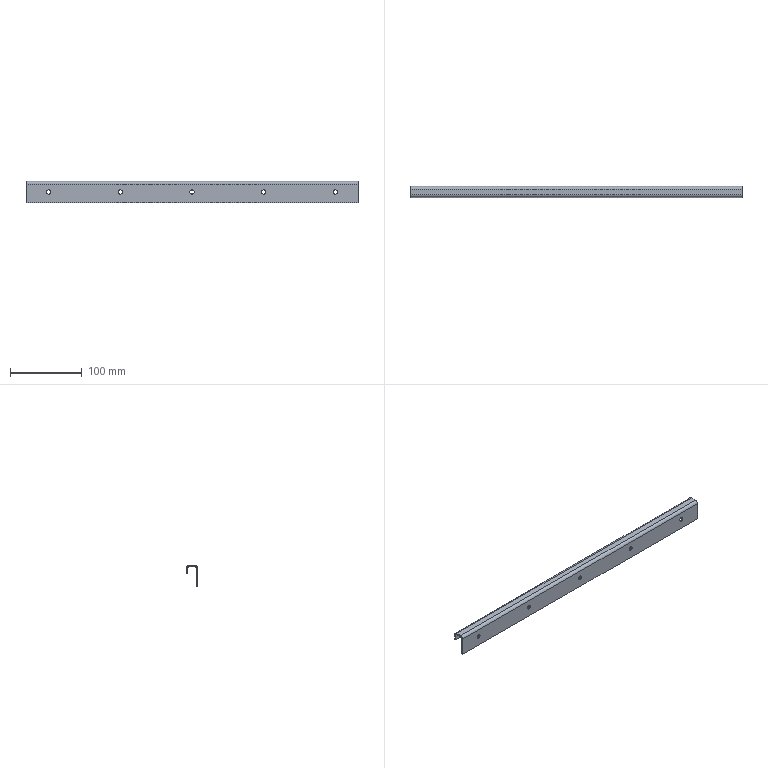Part | NX | features solid 2 | 1 solid | 24 faces | box 463 x 15.5 x 30 mm | volume 46874 mm3 | cylinder 14 | plane 10 | commonest cylinder face diameters 6 x10 4 x2 8 x2
STEP:
#1=CARTESIAN_POINT('',(773.5,-1576.,350.));
#2=VERTEX_POINT('',#1);
#3=CARTESIAN_POINT('',(773.5,-1578.,350.));
#4=VERTEX_POINT('',#3);
#5=CARTESIAN_POINT('',(773.5,-2040.23,350.));
#6=DIRECTION('',(0.,1.,0.));
#7=VECTOR('',#6,1000.);
#8=LINE('',#5,#7);
#9=EDGE_CURVE('',#2,#4,#8,.F.);
#10=ORIENTED_EDGE('',*,*,#9,.T.);
#11=CARTESIAN_POINT('',(773.5,-1578.,356.));
#12=VERTEX_POINT('',#11);
#13=CARTESIAN_POINT('',(773.5,-1578.,353.));
#14=DIRECTION('',(0.,-1.,0.));
#15=DIRECTION('',(0.,0.,-1.));
#16=AXIS2_PLACEMENT_3D('',#13,#14,#15);
#17=CIRCLE('',#16,3.);
#18=EDGE_CURVE('',#4,#12,#17,.T.);
#19=ORIENTED_EDGE('',*,*,#18,.T.);
#20=CARTESIAN_POINT('',(773.5,-1576.,356.));
#21=VERTEX_POINT('',#20);
#22=CARTESIAN_POINT('',(773.5,-2040.23,356.));
#23=DIRECTION('',(0.,1.,0.));
#24=VECTOR('',#23,1000.);
#25=LINE('',#22,#24);
#26=EDGE_CURVE('',#12,#21,#25,.T.);
#27=ORIENTED_EDGE('',*,*,#26,.T.);
#28=CARTESIAN_POINT('',(773.5,-1576.,353.));
#29=DIRECTION('',(0.,1.,0.));
#30=DIRECTION('',(-1.,0.,0.));
#31=AXIS2_PLACEMENT_3D('',#28,#29,#30);
#32=CIRCLE('',#31,3.);
#33=EDGE_CURVE('',#21,#2,#32,.T.);
#34=ORIENTED_EDGE('',*,*,#33,.T.);
#35=EDGE_LOOP('',(#10,#19,#27,#34));
#36=FACE_BOUND('',#35,.T.);
#37=CARTESIAN_POINT('',(773.5,-2040.23,353.));
#38=DIRECTION('',(0.,1.,0.));
#39=DIRECTION('',(0.,0.,1.));
#40=AXIS2_PLACEMENT_3D('',#37,#38,#39);
#41=CYLINDRICAL_SURFACE('',#40,3.);
#42=ADVANCED_FACE('',(#36),#41,.F.);
#43=CARTESIAN_POINT('',(973.5,-1576.,350.));
#44=VERTEX_POINT('',#43);
#45=CARTESIAN_POINT('',(973.5,-1578.,350.));
#46=VERTEX_POINT('',#45);
#47=CARTESIAN_POINT('',(973.5,-2040.23,350.));
#48=DIRECTION('',(0.,1.,0.));
#49=VECTOR('',#48,1000.);
#50=LINE('',#47,#49);
#51=EDGE_CURVE('',#44,#46,#50,.F.);
#52=ORIENTED_EDGE('',*,*,#51,.T.);
#53=CARTESIAN_POINT('',(973.5,-1578.,356.));
#54=VERTEX_POINT('',#53);
#55=CARTESIAN_POINT('',(973.5,-1578.,353.));
#56=DIRECTION('',(0.,-1.,0.));
#57=DIRECTION('',(0.,0.,-1.));
#58=AXIS2_PLACEMENT_3D('',#55,#56,#57);
#59=CIRCLE('',#58,3.);
#60=EDGE_CURVE('',#46,#54,#59,.T.);
#61=ORIENTED_EDGE('',*,*,#60,.T.);
#62=CARTESIAN_POINT('',(973.5,-1576.,356.));
#63=VERTEX_POINT('',#62);
#64=CARTESIAN_POINT('',(973.5,-2040.23,356.));
#65=DIRECTION('',(0.,1.,0.));
#66=VECTOR('',#65,1000.);
#67=LINE('',#64,#66);
#68=EDGE_CURVE('',#54,#63,#67,.T.);
#69=ORIENTED_EDGE('',*,*,#68,.T.);
#70=CARTESIAN_POINT('',(973.5,-1576.,353.));
#71=DIRECTION('',(0.,1.,0.));
#72=DIRECTION('',(-1.,0.,0.));
#73=AXIS2_PLACEMENT_3D('',#70,#71,#72);
#74=CIRCLE('',#73,3.);
#75=EDGE_CURVE('',#63,#44,#74,.T.);
#76=ORIENTED_EDGE('',*,*,#75,.T.);
#77=EDGE_LOOP('',(#52,#61,#69,#76));
#78=FACE_BOUND('',#77,.T.);
#79=CARTESIAN_POINT('',(973.5,-2040.23,353.));
#80=DIRECTION('',(0.,1.,0.));
#81=DIRECTION('',(0.,0.,1.));
#82=AXIS2_PLACEMENT_3D('',#79,#80,#81);
#83=CYLINDRICAL_SURFACE('',#82,3.);
#84=ADVANCED_FACE('',(#78),#83,.F.);
#85=CARTESIAN_POINT('',(873.5,-1576.,350.));
#86=VERTEX_POINT('',#85);
#87=CARTESIAN_POINT('',(873.5,-1578.,350.));
#88=VERTEX_POINT('',#87);
#89=CARTESIAN_POINT('',(873.5,-2040.23,350.));
#90=DIRECTION('',(0.,1.,0.));
#91=VECTOR('',#90,1000.);
#92=LINE('',#89,#91);
#93=EDGE_CURVE('',#86,#88,#92,.F.);
#94=ORIENTED_EDGE('',*,*,#93,.T.);
#95=CARTESIAN_POINT('',(873.5,-1578.,356.));
#96=VERTEX_POINT('',#95);
#97=CARTESIAN_POINT('',(873.5,-1578.,353.));
#98=DIRECTION('',(0.,-1.,0.));
#99=DIRECTION('',(0.,0.,-1.));
#100=AXIS2_PLACEMENT_3D('',#97,#98,#99);
#101=CIRCLE('',#100,3.);
#102=EDGE_CURVE('',#88,#96,#101,.T.);
#103=ORIENTED_EDGE('',*,*,#102,.T.);
#104=CARTESIAN_POINT('',(873.5,-1576.,356.));
#105=VERTEX_POINT('',#104);
#106=CARTESIAN_POINT('',(873.5,-2040.23,356.));
#107=DIRECTION('',(0.,1.,0.));
#108=VECTOR('',#107,1000.);
#109=LINE('',#106,#108);
#110=EDGE_CURVE('',#96,#105,#109,.T.);
#111=ORIENTED_EDGE('',*,*,#110,.T.);
#112=CARTESIAN_POINT('',(873.5,-1576.,353.));
#113=DIRECTION('',(0.,1.,0.));
#114=DIRECTION('',(-1.,0.,0.));
#115=AXIS2_PLACEMENT_3D('',#112,#113,#114);
#116=CIRCLE('',#115,3.);
#117=EDGE_CURVE('',#105,#86,#116,.T.);
#118=ORIENTED_EDGE('',*,*,#117,.T.);
#119=EDGE_LOOP('',(#94,#103,#111,#118));
#120=FACE_BOUND('',#119,.T.);
#121=CARTESIAN_POINT('',(873.5,-2040.23,353.));
#122=DIRECTION('',(0.,1.,0.));
#123=DIRECTION('',(0.,0.,1.));
#124=AXIS2_PLACEMENT_3D('',#121,#122,#123);
#125=CYLINDRICAL_SURFACE('',#124,3.);
#126=ADVANCED_FACE('',(#120),#125,.F.);
#127=CARTESIAN_POINT('',(573.5,-1576.,350.));
#128=VERTEX_POINT('',#127);
#129=CARTESIAN_POINT('',(573.5,-1578.,350.));
#130=VERTEX_POINT('',#129);
#131=CARTESIAN_POINT('',(573.5,-2040.23,350.));
#132=DIRECTION('',(0.,1.,0.));
#133=VECTOR('',#132,1000.);
#134=LINE('',#131,#133);
#135=EDGE_CURVE('',#128,#130,#134,.F.);
#136=ORIENTED_EDGE('',*,*,#135,.T.);
#137=CARTESIAN_POINT('',(573.5,-1578.,356.));
#138=VERTEX_POINT('',#137);
#139=CARTESIAN_POINT('',(573.5,-1578.,353.));
#140=DIRECTION('',(0.,-1.,0.));
#141=DIRECTION('',(0.,0.,-1.));
#142=AXIS2_PLACEMENT_3D('',#139,#140,#141);
#143=CIRCLE('',#142,3.);
#144=EDGE_CURVE('',#130,#138,#143,.T.);
#145=ORIENTED_EDGE('',*,*,#144,.T.);
#146=CARTESIAN_POINT('',(573.5,-1576.,356.));
#147=VERTEX_POINT('',#146);
#148=CARTESIAN_POINT('',(573.5,-2040.23,356.));
#149=DIRECTION('',(0.,1.,0.));
#150=VECTOR('',#149,1000.);
#151=LINE('',#148,#150);
#152=EDGE_CURVE('',#138,#147,#151,.T.);
#153=ORIENTED_EDGE('',*,*,#152,.T.);
#154=CARTESIAN_POINT('',(573.5,-1576.,353.));
#155=DIRECTION('',(0.,1.,0.));
#156=DIRECTION('',(-1.,0.,0.));
#157=AXIS2_PLACEMENT_3D('',#154,#155,#156);
#158=CIRCLE('',#157,3.);
#159=EDGE_CURVE('',#147,#128,#158,.T.);
#160=ORIENTED_EDGE('',*,*,#159,.T.);
#161=EDGE_LOOP('',(#136,#145,#153,#160));
#162=FACE_BOUND('',#161,.T.);
#163=CARTESIAN_POINT('',(573.5,-2040.23,353.));
#164=DIRECTION('',(0.,1.,0.));
#165=DIRECTION('',(0.,0.,1.));
#166=AXIS2_PLACEMENT_3D('',#163,#164,#165);
#167=CYLINDRICAL_SURFACE('',#166,3.);
#168=ADVANCED_FACE('',(#162),#167,.F.);
#169=CARTESIAN_POINT('',(673.5,-1576.,350.));
#170=VERTEX_POINT('',#169);
#171=CARTESIAN_POINT('',(673.5,-1578.,350.));
#172=VERTEX_POINT('',#171);
#173=CARTESIAN_POINT('',(673.5,-2040.23,350.));
#174=DIRECTION('',(0.,1.,0.));
#175=VECTOR('',#174,1000.);
#176=LINE('',#173,#175);
#177=EDGE_CURVE('',#170,#172,#176,.F.);
#178=ORIENTED_EDGE('',*,*,#177,.T.);
#179=CARTESIAN_POINT('',(673.5,-1578.,356.));
#180=VERTEX_POINT('',#179);
#181=CARTESIAN_POINT('',(673.5,-1578.,353.));
#182=DIRECTION('',(0.,-1.,0.));
#183=DIRECTION('',(0.,0.,-1.));
#184=AXIS2_PLACEMENT_3D('',#181,#182,#183);
#185=CIRCLE('',#184,3.);
#186=EDGE_CURVE('',#172,#180,#185,.T.);
#187=ORIENTED_EDGE('',*,*,#186,.T.);
#188=CARTESIAN_POINT('',(673.5,-1576.,356.));
#189=VERTEX_POINT('',#188);
#190=CARTESIAN_POINT('',(673.5,-2040.23,356.));
#191=DIRECTION('',(0.,1.,0.));
#192=VECTOR('',#191,1000.);
#193=LINE('',#190,#192);
#194=EDGE_CURVE('',#180,#189,#193,.T.);
#195=ORIENTED_EDGE('',*,*,#194,.T.);
#196=CARTESIAN_POINT('',(673.5,-1576.,353.));
#197=DIRECTION('',(0.,1.,0.));
#198=DIRECTION('',(-1.,0.,0.));
#199=AXIS2_PLACEMENT_3D('',#196,#197,#198);
#200=CIRCLE('',#199,3.);
#201=EDGE_CURVE('',#189,#170,#200,.T.);
#202=ORIENTED_EDGE('',*,*,#201,.T.);
#203=EDGE_LOOP('',(#178,#187,#195,#202));
#204=FACE_BOUND('',#203,.T.);
#205=CARTESIAN_POINT('',(673.5,-2040.23,353.));
#206=DIRECTION('',(0.,1.,0.));
#207=DIRECTION('',(0.,0.,1.));
#208=AXIS2_PLACEMENT_3D('',#205,#206,#207);
#209=CYLINDRICAL_SURFACE('',#208,3.);
#210=ADVANCED_FACE('',(#204),#209,.F.);
#211=CARTESIAN_POINT('',(542.,-1564.5,364.));
#212=VERTEX_POINT('',#211);
#213=CARTESIAN_POINT('',(542.,-1564.5,356.));
#214=VERTEX_POINT('',#213);
#215=CARTESIAN_POINT('',(542.,-1564.5,368.));
#216=DIRECTION('',(0.,0.,-1.));
#217=VECTOR('',#216,1000.);
#218=LINE('',#215,#217);
#219=EDGE_CURVE('',#212,#214,#218,.T.);
#220=ORIENTED_EDGE('',*,*,#219,.T.);
#221=CARTESIAN_POINT('',(1005.,-1564.5,356.));
#222=VERTEX_POINT('',#221);
#223=CARTESIAN_POINT('',(1005.,-1564.5,356.));
#224=DIRECTION('',(-1.,0.,0.));
#225=VECTOR('',#224,1000.);
#226=LINE('',#223,#225);
#227=EDGE_CURVE('',#222,#214,#226,.T.);
#228=ORIENTED_EDGE('',*,*,#227,.F.);
#229=CARTESIAN_POINT('',(1005.,-1564.5,364.));
#230=VERTEX_POINT('',#229);
#231=CARTESIAN_POINT('',(1005.,-1564.5,368.));
#232=DIRECTION('',(0.,0.,-1.));
#233=VECTOR('',#232,1000.);
#234=LINE('',#231,#233);
#235=EDGE_CURVE('',#230,#222,#234,.T.);
#236=ORIENTED_EDGE('',*,*,#235,.F.);
#237=CARTESIAN_POINT('',(1005.,-1564.5,364.));
#238=DIRECTION('',(-1.,0.,0.));
#239=VECTOR('',#238,1000.);
#240=LINE('',#237,#239);
#241=EDGE_CURVE('',#230,#212,#240,.T.);
#242=ORIENTED_EDGE('',*,*,#241,.T.);
#243=EDGE_LOOP('',(#220,#228,#236,#242));
#244=FACE_BOUND('',#243,.T.);
#245=CARTESIAN_POINT('',(1005.,-1564.5,368.));
#246=DIRECTION('',(0.,1.,0.));
#247=DIRECTION('',(0.,0.,-1.));
#248=AXIS2_PLACEMENT_3D('',#245,#246,#247);
#249=PLANE('',#248);
#250=ADVANCED_FACE('',(#244),#249,.F.);
#251=CARTESIAN_POINT('',(542.,-1566.5,366.));
#252=VERTEX_POINT('',#251);
#253=CARTESIAN_POINT('',(542.,-1566.5,364.));
#254=DIRECTION('',(-1.,0.,0.));
#255=DIRECTION('',(0.,0.,-1.));
#256=AXIS2_PLACEMENT_3D('',#253,#254,#255);
#257=CIRCLE('',#256,2.);
#258=EDGE_CURVE('',#252,#212,#257,.T.);
#259=ORIENTED_EDGE('',*,*,#258,.T.);
#260=ORIENTED_EDGE('',*,*,#241,.F.);
#261=CARTESIAN_POINT('',(1005.,-1566.5,366.));
#262=VERTEX_POINT('',#261);
#263=CARTESIAN_POINT('',(1005.,-1566.5,364.));
#264=DIRECTION('',(-1.,0.,0.));
#265=DIRECTION('',(0.,0.,-1.));
#266=AXIS2_PLACEMENT_3D('',#263,#264,#265);
#267=CIRCLE('',#266,2.);
#268=EDGE_CURVE('',#262,#230,#267,.T.);
#269=ORIENTED_EDGE('',*,*,#268,.F.);
#270=CARTESIAN_POINT('',(1005.,-1566.5,366.));
#271=DIRECTION('',(-1.,0.,0.));
#272=VECTOR('',#271,1000.);
#273=LINE('',#270,#272);
#274=EDGE_CURVE('',#262,#252,#273,.T.);
#275=ORIENTED_EDGE('',*,*,#274,.T.);
#276=EDGE_LOOP('',(#259,#260,#269,#275));
#277=FACE_BOUND('',#276,.T.);
#278=CARTESIAN_POINT('',(1005.,-1566.5,364.));
#279=DIRECTION('',(-1.,0.,0.));
#280=DIRECTION('',(0.,0.,-1.));
#281=AXIS2_PLACEMENT_3D('',#278,#279,#280);
#282=CYLINDRICAL_SURFACE('',#281,2.);
#283=ADVANCED_FACE('',(#277),#282,.F.);
#284=CARTESIAN_POINT('',(542.,-1574.,366.));
#285=VERTEX_POINT('',#284);
#286=CARTESIAN_POINT('',(542.,-1578.,366.));
#287=DIRECTION('',(0.,1.,0.));
#288=VECTOR('',#287,1000.);
#289=LINE('',#286,#288);
#290=EDGE_CURVE('',#285,#252,#289,.T.);
#291=ORIENTED_EDGE('',*,*,#290,.T.);
#292=ORIENTED_EDGE('',*,*,#274,.F.);
#293=CARTESIAN_POINT('',(1005.,-1574.,366.));
#294=VERTEX_POINT('',#293);
#295=CARTESIAN_POINT('',(1005.,-1578.,366.));
#296=DIRECTION('',(0.,1.,0.));
#297=VECTOR('',#296,1000.);
#298=LINE('',#295,#297);
#299=EDGE_CURVE('',#294,#262,#298,.T.);
#300=ORIENTED_EDGE('',*,*,#299,.F.);
#301=CARTESIAN_POINT('',(1005.,-1574.,366.));
#302=DIRECTION('',(-1.,0.,0.));
#303=VECTOR('',#302,1000.);
#304=LINE('',#301,#303);
#305=EDGE_CURVE('',#294,#285,#304,.T.);
#306=ORIENTED_EDGE('',*,*,#305,.T.);
#307=EDGE_LOOP('',(#291,#292,#300,#306));
#308=FACE_BOUND('',#307,.T.);
#309=CARTESIAN_POINT('',(1005.,-1578.,366.));
#310=DIRECTION('',(0.,0.,1.));
#311=DIRECTION('',(0.,-1.,0.));
#312=AXIS2_PLACEMENT_3D('',#309,#310,#311);
#313=PLANE('',#312);
#314=ADVANCED_FACE('',(#308),#313,.F.);
#315=CARTESIAN_POINT('',(542.,-1576.,364.));
#316=VERTEX_POINT('',#315);
#317=CARTESIAN_POINT('',(542.,-1574.,364.));
#318=DIRECTION('',(-1.,0.,0.));
#319=DIRECTION('',(0.,0.,-1.));
#320=AXIS2_PLACEMENT_3D('',#317,#318,#319);
#321=CIRCLE('',#320,2.);
#322=EDGE_CURVE('',#316,#285,#321,.T.);
#323=ORIENTED_EDGE('',*,*,#322,.T.);
#324=ORIENTED_EDGE('',*,*,#305,.F.);
#325=CARTESIAN_POINT('',(1005.,-1576.,364.));
#326=VERTEX_POINT('',#325);
#327=CARTESIAN_POINT('',(1005.,-1574.,364.));
#328=DIRECTION('',(-1.,0.,0.));
#329=DIRECTION('',(0.,0.,-1.));
#330=AXIS2_PLACEMENT_3D('',#327,#328,#329);
#331=CIRCLE('',#330,2.);
#332=EDGE_CURVE('',#326,#294,#331,.T.);
#333=ORIENTED_EDGE('',*,*,#332,.F.);
#334=CARTESIAN_POINT('',(1005.,-1576.,364.));
#335=DIRECTION('',(-1.,0.,0.));
#336=VECTOR('',#335,1000.);
#337=LINE('',#334,#336);
#338=EDGE_CURVE('',#326,#316,#337,.T.);
#339=ORIENTED_EDGE('',*,*,#338,.T.);
#340=EDGE_LOOP('',(#323,#324,#333,#339));
#341=FACE_BOUND('',#340,.T.);
#342=CARTESIAN_POINT('',(1005.,-1574.,364.));
#343=DIRECTION('',(-1.,0.,0.));
#344=DIRECTION('',(0.,0.,-1.));
#345=AXIS2_PLACEMENT_3D('',#342,#343,#344);
#346=CYLINDRICAL_SURFACE('',#345,2.);
#347=ADVANCED_FACE('',(#341),#346,.F.);
#348=ORIENTED_EDGE('',*,*,#201,.F.);
#349=CARTESIAN_POINT('',(673.5,-1576.,353.));
#350=DIRECTION('',(0.,1.,0.));
#351=DIRECTION('',(-1.,0.,0.));
#352=AXIS2_PLACEMENT_3D('',#349,#350,#351);
#353=CIRCLE('',#352,3.);
#354=EDGE_CURVE('',#170,#189,#353,.T.);
#355=ORIENTED_EDGE('',*,*,#354,.F.);
#356=EDGE_LOOP('',(#348,#355));
#357=FACE_BOUND('',#356,.T.);
#358=ORIENTED_EDGE('',*,*,#159,.F.);
#359=CARTESIAN_POINT('',(573.5,-1576.,353.));
#360=DIRECTION('',(0.,1.,0.));
#361=DIRECTION('',(-1.,0.,0.));
#362=AXIS2_PLACEMENT_3D('',#359,#360,#361);
#363=CIRCLE('',#362,3.);
#364=EDGE_CURVE('',#128,#147,#363,.T.);
#365=ORIENTED_EDGE('',*,*,#364,.F.);
#366=EDGE_LOOP('',(#358,#365));
#367=FACE_BOUND('',#366,.T.);
#368=ORIENTED_EDGE('',*,*,#117,.F.);
#369=CARTESIAN_POINT('',(873.5,-1576.,353.));
#370=DIRECTION('',(0.,1.,0.));
#371=DIRECTION('',(-1.,0.,0.));
#372=AXIS2_PLACEMENT_3D('',#369,#370,#371);
#373=CIRCLE('',#372,3.);
#374=EDGE_CURVE('',#86,#105,#373,.T.);
#375=ORIENTED_EDGE('',*,*,#374,.F.);
#376=EDGE_LOOP('',(#368,#375));
#377=FACE_BOUND('',#376,.T.);
#378=ORIENTED_EDGE('',*,*,#75,.F.);
#379=CARTESIAN_POINT('',(973.5,-1576.,353.));
#380=DIRECTION('',(0.,1.,0.));
#381=DIRECTION('',(-1.,0.,0.));
#382=AXIS2_PLACEMENT_3D('',#379,#380,#381);
#383=CIRCLE('',#382,3.);
#384=EDGE_CURVE('',#44,#63,#383,.T.);
#385=ORIENTED_EDGE('',*,*,#384,.F.);
#386=EDGE_LOOP('',(#378,#385));
#387=FACE_BOUND('',#386,.T.);
#388=ORIENTED_EDGE('',*,*,#33,.F.);
#389=CARTESIAN_POINT('',(773.5,-1576.,353.));
#390=DIRECTION('',(0.,1.,0.));
#391=DIRECTION('',(-1.,0.,0.));
#392=AXIS2_PLACEMENT_3D('',#389,#390,#391);
#393=CIRCLE('',#392,3.);
#394=EDGE_CURVE('',#2,#21,#393,.T.);
#395=ORIENTED_EDGE('',*,*,#394,.F.);
#396=EDGE_LOOP('',(#388,#395));
#397=FACE_BOUND('',#396,.T.);
#398=CARTESIAN_POINT('',(542.,-1576.,338.));
#399=VERTEX_POINT('',#398);
#400=CARTESIAN_POINT('',(542.,-1576.,338.));
#401=DIRECTION('',(0.,0.,1.));
#402=VECTOR('',#401,1000.);
#403=LINE('',#400,#402);
#404=EDGE_CURVE('',#399,#316,#403,.T.);
#405=ORIENTED_EDGE('',*,*,#404,.T.);
#406=ORIENTED_EDGE('',*,*,#338,.F.);
#407=CARTESIAN_POINT('',(1005.,-1576.,338.));
#408=VERTEX_POINT('',#407);
#409=CARTESIAN_POINT('',(1005.,-1576.,338.));
#410=DIRECTION('',(0.,0.,1.));
#411=VECTOR('',#410,1000.);
#412=LINE('',#409,#411);
#413=EDGE_CURVE('',#408,#326,#412,.T.);
#414=ORIENTED_EDGE('',*,*,#413,.F.);
#415=CARTESIAN_POINT('',(1005.,-1576.,338.));
#416=DIRECTION('',(-1.,0.,0.));
#417=VECTOR('',#416,1000.);
#418=LINE('',#415,#417);
#419=EDGE_CURVE('',#408,#399,#418,.T.);
#420=ORIENTED_EDGE('',*,*,#419,.T.);
#421=EDGE_LOOP('',(#405,#406,#414,#420));
#422=FACE_BOUND('',#421,.T.);
#423=CARTESIAN_POINT('',(1005.,-1576.,338.));
#424=DIRECTION('',(0.,-1.,0.));
#425=DIRECTION('',(-1.,0.,0.));
#426=AXIS2_PLACEMENT_3D('',#423,#424,#425);
#427=PLANE('',#426);
#428=ADVANCED_FACE('',(#357,#367,#377,#387,#397,#422),#427,.F.);
#429=CARTESIAN_POINT('',(542.,-1562.5,364.));
#430=VERTEX_POINT('',#429);
#431=CARTESIAN_POINT('',(542.,-1562.5,356.));
#432=VERTEX_POINT('',#431);
#433=CARTESIAN_POINT('',(542.,-1562.5,368.));
#434=DIRECTION('',(0.,0.,-1.));
#435=VECTOR('',#434,1000.);
#436=LINE('',#433,#435);
#437=EDGE_CURVE('',#430,#432,#436,.T.);
#438=ORIENTED_EDGE('',*,*,#437,.F.);
#439=CARTESIAN_POINT('',(1005.,-1562.5,364.));
#440=VERTEX_POINT('',#439);
#441=CARTESIAN_POINT('',(1005.,-1562.5,364.));
#442=DIRECTION('',(-1.,0.,0.));
#443=VECTOR('',#442,1000.);
#444=LINE('',#441,#443);
#445=EDGE_CURVE('',#440,#430,#444,.T.);
#446=ORIENTED_EDGE('',*,*,#445,.F.);
#447=CARTESIAN_POINT('',(1005.,-1562.5,356.));
#448=VERTEX_POINT('',#447);
#449=CARTESIAN_POINT('',(1005.,-1562.5,368.));
#450=DIRECTION('',(0.,0.,-1.));
#451=VECTOR('',#450,1000.);
#452=LINE('',#449,#451);
#453=EDGE_CURVE('',#440,#448,#452,.T.);
#454=ORIENTED_EDGE('',*,*,#453,.T.);
#455=CARTESIAN_POINT('',(1005.,-1562.5,356.));
#456=DIRECTION('',(-1.,0.,0.));
#457=VECTOR('',#456,1000.);
#458=LINE('',#455,#457);
#459=EDGE_CURVE('',#448,#432,#458,.T.);
#460=ORIENTED_EDGE('',*,*,#459,.T.);
#461=EDGE_LOOP('',(#438,#446,#454,#460));
#462=FACE_BOUND('',#461,.T.);
#463=CARTESIAN_POINT('',(1005.,-1562.5,368.));
#464=DIRECTION('',(0.,1.,0.));
#465=DIRECTION('',(0.,0.,-1.));
#466=AXIS2_PLACEMENT_3D('',#463,#464,#465);
#467=PLANE('',#466);
#468=ADVANCED_FACE('',(#462),#467,.T.);
#469=CARTESIAN_POINT('',(542.,-1566.5,368.));
#470=VERTEX_POINT('',#469);
#471=CARTESIAN_POINT('',(542.,-1566.5,364.));
#472=DIRECTION('',(-1.,0.,0.));
#473=DIRECTION('',(0.,0.,1.));
#474=AXIS2_PLACEMENT_3D('',#471,#472,#473);
#475=CIRCLE('',#474,4.);
#476=EDGE_CURVE('',#470,#430,#475,.T.);
#477=ORIENTED_EDGE('',*,*,#476,.F.);
#478=CARTESIAN_POINT('',(1005.,-1566.5,368.));
#479=VERTEX_POINT('',#478);
#480=CARTESIAN_POINT('',(1005.,-1566.5,368.));
#481=DIRECTION('',(-1.,0.,0.));
#482=VECTOR('',#481,1000.);
#483=LINE('',#480,#482);
#484=EDGE_CURVE('',#479,#470,#483,.T.);
#485=ORIENTED_EDGE('',*,*,#484,.F.);
#486=CARTESIAN_POINT('',(1005.,-1566.5,364.));
#487=DIRECTION('',(-1.,0.,0.));
#488=DIRECTION('',(0.,0.,1.));
#489=AXIS2_PLACEMENT_3D('',#486,#487,#488);
#490=CIRCLE('',#489,4.);
#491=EDGE_CURVE('',#479,#440,#490,.T.);
#492=ORIENTED_EDGE('',*,*,#491,.T.);
#493=ORIENTED_EDGE('',*,*,#445,.T.);
#494=EDGE_LOOP('',(#477,#485,#492,#493));
#495=FACE_BOUND('',#494,.T.);
#496=CARTESIAN_POINT('',(1005.,-1566.5,364.));
#497=DIRECTION('',(-1.,0.,0.));
#498=DIRECTION('',(0.,0.,-1.));
#499=AXIS2_PLACEMENT_3D('',#496,#497,#498);
#500=CYLINDRICAL_SURFACE('',#499,4.);
#501=ADVANCED_FACE('',(#495),#500,.T.);
#502=CARTESIAN_POINT('',(542.,-1574.,368.));
#503=VERTEX_POINT('',#502);
#504=CARTESIAN_POINT('',(542.,-1578.,368.));
#505=DIRECTION('',(0.,1.,0.));
#506=VECTOR('',#505,1000.);
#507=LINE('',#504,#506);
#508=EDGE_CURVE('',#503,#470,#507,.T.);
#509=ORIENTED_EDGE('',*,*,#508,.F.);
#510=CARTESIAN_POINT('',(1005.,-1574.,368.));
#511=VERTEX_POINT('',#510);
#512=CARTESIAN_POINT('',(1005.,-1574.,368.));
#513=DIRECTION('',(-1.,0.,0.));
#514=VECTOR('',#513,1000.);
#515=LINE('',#512,#514);
#516=EDGE_CURVE('',#511,#503,#515,.T.);
#517=ORIENTED_EDGE('',*,*,#516,.F.);
#518=CARTESIAN_POINT('',(1005.,-1578.,368.));
#519=DIRECTION('',(0.,1.,0.));
#520=VECTOR('',#519,1000.);
#521=LINE('',#518,#520);
#522=EDGE_CURVE('',#511,#479,#521,.T.);
#523=ORIENTED_EDGE('',*,*,#522,.T.);
#524=ORIENTED_EDGE('',*,*,#484,.T.);
#525=EDGE_LOOP('',(#509,#517,#523,#524));
#526=FACE_BOUND('',#525,.T.);
#527=CARTESIAN_POINT('',(1005.,-1578.,368.));
#528=DIRECTION('',(0.,0.,1.));
#529=DIRECTION('',(0.,-1.,0.));
#530=AXIS2_PLACEMENT_3D('',#527,#528,#529);
#531=PLANE('',#530);
#532=ADVANCED_FACE('',(#526),#531,.T.);
#533=CARTESIAN_POINT('',(542.,-1578.,364.));
#534=VERTEX_POINT('',#533);
#535=CARTESIAN_POINT('',(542.,-1574.,364.));
#536=DIRECTION('',(-1.,0.,0.));
#537=DIRECTION('',(0.,0.,1.));
#538=AXIS2_PLACEMENT_3D('',#535,#536,#537);
#539=CIRCLE('',#538,4.);
#540=EDGE_CURVE('',#534,#503,#539,.T.);
#541=ORIENTED_EDGE('',*,*,#540,.F.);
#542=CARTESIAN_POINT('',(1005.,-1578.,364.));
#543=VERTEX_POINT('',#542);
#544=CARTESIAN_POINT('',(1005.,-1578.,364.));
#545=DIRECTION('',(-1.,0.,0.));
#546=VECTOR('',#545,1000.);
#547=LINE('',#544,#546);
#548=EDGE_CURVE('',#543,#534,#547,.T.);
#549=ORIENTED_EDGE('',*,*,#548,.F.);
#550=CARTESIAN_POINT('',(1005.,-1574.,364.));
#551=DIRECTION('',(-1.,0.,0.));
#552=DIRECTION('',(0.,0.,1.));
#553=AXIS2_PLACEMENT_3D('',#550,#551,#552);
#554=CIRCLE('',#553,4.);
#555=EDGE_CURVE('',#543,#511,#554,.T.);
#556=ORIENTED_EDGE('',*,*,#555,.T.);
#557=ORIENTED_EDGE('',*,*,#516,.T.);
#558=EDGE_LOOP('',(#541,#549,#556,#557));
#559=FACE_BOUND('',#558,.T.);
#560=CARTESIAN_POINT('',(1005.,-1574.,364.));
#561=DIRECTION('',(-1.,0.,0.));
#562=DIRECTION('',(0.,0.,-1.));
#563=AXIS2_PLACEMENT_3D('',#560,#561,#562);
#564=CYLINDRICAL_SURFACE('',#563,4.);
#565=ADVANCED_FACE('',(#559),#564,.T.);
#566=CARTESIAN_POINT('',(673.5,-1578.,353.));
#567=DIRECTION('',(0.,-1.,0.));
#568=DIRECTION('',(0.,0.,-1.));
#569=AXIS2_PLACEMENT_3D('',#566,#567,#568);
#570=CIRCLE('',#569,3.);
#571=EDGE_CURVE('',#180,#172,#570,.T.);
#572=ORIENTED_EDGE('',*,*,#571,.F.);
#573=ORIENTED_EDGE('',*,*,#186,.F.);
#574=EDGE_LOOP('',(#572,#573));
#575=FACE_BOUND('',#574,.T.);
#576=CARTESIAN_POINT('',(573.5,-1578.,353.));
#577=DIRECTION('',(0.,-1.,0.));
#578=DIRECTION('',(0.,0.,-1.));
#579=AXIS2_PLACEMENT_3D('',#576,#577,#578);
#580=CIRCLE('',#579,3.);
#581=EDGE_CURVE('',#138,#130,#580,.T.);
#582=ORIENTED_EDGE('',*,*,#581,.F.);
#583=ORIENTED_EDGE('',*,*,#144,.F.);
#584=EDGE_LOOP('',(#582,#583));
#585=FACE_BOUND('',#584,.T.);
#586=CARTESIAN_POINT('',(873.5,-1578.,353.));
#587=DIRECTION('',(0.,-1.,0.));
#588=DIRECTION('',(0.,0.,-1.));
#589=AXIS2_PLACEMENT_3D('',#586,#587,#588);
#590=CIRCLE('',#589,3.);
#591=EDGE_CURVE('',#96,#88,#590,.T.);
#592=ORIENTED_EDGE('',*,*,#591,.F.);
#593=ORIENTED_EDGE('',*,*,#102,.F.);
#594=EDGE_LOOP('',(#592,#593));
#595=FACE_BOUND('',#594,.T.);
#596=CARTESIAN_POINT('',(973.5,-1578.,353.));
#597=DIRECTION('',(0.,-1.,0.));
#598=DIRECTION('',(0.,0.,-1.));
#599=AXIS2_PLACEMENT_3D('',#596,#597,#598);
#600=CIRCLE('',#599,3.);
#601=EDGE_CURVE('',#54,#46,#600,.T.);
#602=ORIENTED_EDGE('',*,*,#601,.F.);
#603=ORIENTED_EDGE('',*,*,#60,.F.);
#604=EDGE_LOOP('',(#602,#603));
#605=FACE_BOUND('',#604,.T.);
#606=CARTESIAN_POINT('',(773.5,-1578.,353.));
#607=DIRECTION('',(0.,-1.,0.));
#608=DIRECTION('',(0.,0.,-1.));
#609=AXIS2_PLACEMENT_3D('',#606,#607,#608);
#610=CIRCLE('',#609,3.);
#611=EDGE_CURVE('',#12,#4,#610,.T.);
#612=ORIENTED_EDGE('',*,*,#611,.F.);
#613=ORIENTED_EDGE('',*,*,#18,.F.);
#614=EDGE_LOOP('',(#612,#613));
#615=FACE_BOUND('',#614,.T.);
#616=CARTESIAN_POINT('',(542.,-1578.,338.));
#617=VERTEX_POINT('',#616);
#618=CARTESIAN_POINT('',(542.,-1578.,338.));
#619=DIRECTION('',(0.,0.,1.));
#620=VECTOR('',#619,1000.);
#621=LINE('',#618,#620);
#622=EDGE_CURVE('',#617,#534,#621,.T.);
#623=ORIENTED_EDGE('',*,*,#622,.F.);
#624=CARTESIAN_POINT('',(1005.,-1578.,338.));
#625=VERTEX_POINT('',#624);
#626=CARTESIAN_POINT('',(1005.,-1578.,338.));
#627=DIRECTION('',(-1.,0.,0.));
#628=VECTOR('',#627,1000.);
#629=LINE('',#626,#628);
#630=EDGE_CURVE('',#625,#617,#629,.T.);
#631=ORIENTED_EDGE('',*,*,#630,.F.);
#632=CARTESIAN_POINT('',(1005.,-1578.,338.));
#633=DIRECTION('',(0.,0.,1.));
#634=VECTOR('',#633,1000.);
#635=LINE('',#632,#634);
#636=EDGE_CURVE('',#625,#543,#635,.T.);
#637=ORIENTED_EDGE('',*,*,#636,.T.);
#638=ORIENTED_EDGE('',*,*,#548,.T.);
#639=EDGE_LOOP('',(#623,#631,#637,#638));
#640=FACE_BOUND('',#639,.T.);
#641=CARTESIAN_POINT('',(1005.,-1578.,338.));
#642=DIRECTION('',(0.,-1.,0.));
#643=DIRECTION('',(-1.,0.,0.));
#644=AXIS2_PLACEMENT_3D('',#641,#642,#643);
#645=PLANE('',#644);
#646=ADVANCED_FACE('',(#575,#585,#595,#605,#615,#640),#645,.T.);
#647=ORIENTED_EDGE('',*,*,#419,.F.);
#648=CARTESIAN_POINT('',(1005.,-1578.,338.));
#649=DIRECTION('',(0.,-1.,0.));
#650=VECTOR('',#649,1000.);
#651=LINE('',#648,#650);
#652=EDGE_CURVE('',#408,#625,#651,.T.);
#653=ORIENTED_EDGE('',*,*,#652,.T.);
#654=ORIENTED_EDGE('',*,*,#630,.T.);
#655=CARTESIAN_POINT('',(542.,-1578.,338.));
#656=DIRECTION('',(0.,-1.,0.));
#657=VECTOR('',#656,1000.);
#658=LINE('',#655,#657);
#659=EDGE_CURVE('',#399,#617,#658,.T.);
#660=ORIENTED_EDGE('',*,*,#659,.F.);
#661=EDGE_LOOP('',(#647,#653,#654,#660));
#662=FACE_BOUND('',#661,.T.);
#663=CARTESIAN_POINT('',(1005.,-1578.,338.));
#664=DIRECTION('',(0.,0.,1.));
#665=DIRECTION('',(0.,-1.,0.));
#666=AXIS2_PLACEMENT_3D('',#663,#664,#665);
#667=PLANE('',#666);
#668=ADVANCED_FACE('',(#662),#667,.F.);
#669=ORIENTED_EDGE('',*,*,#622,.T.);
#670=ORIENTED_EDGE('',*,*,#540,.T.);
#671=ORIENTED_EDGE('',*,*,#508,.T.);
#672=ORIENTED_EDGE('',*,*,#476,.T.);
#673=ORIENTED_EDGE('',*,*,#437,.T.);
#674=CARTESIAN_POINT('',(542.,-1562.5,356.));
#675=DIRECTION('',(0.,1.,0.));
#676=VECTOR('',#675,1000.);
#677=LINE('',#674,#676);
#678=EDGE_CURVE('',#214,#432,#677,.T.);
#679=ORIENTED_EDGE('',*,*,#678,.F.);
#680=ORIENTED_EDGE('',*,*,#219,.F.);
#681=ORIENTED_EDGE('',*,*,#258,.F.);
#682=ORIENTED_EDGE('',*,*,#290,.F.);
#683=ORIENTED_EDGE('',*,*,#322,.F.);
#684=ORIENTED_EDGE('',*,*,#404,.F.);
#685=ORIENTED_EDGE('',*,*,#659,.T.);
#686=EDGE_LOOP('',(#669,#670,#671,#672,#673,#679,#680,#681,#682,#683,#684,#685));
#687=FACE_BOUND('',#686,.T.);
#688=CARTESIAN_POINT('',(542.,-1578.,338.));
#689=DIRECTION('',(1.,0.,0.));
#690=DIRECTION('',(0.,0.,-1.));
#691=AXIS2_PLACEMENT_3D('',#688,#689,#690);
#692=PLANE('',#691);
#693=ADVANCED_FACE('',(#687),#692,.F.);
#694=CARTESIAN_POINT('',(1005.,-1562.5,356.));
#695=DIRECTION('',(0.,1.,0.));
#696=VECTOR('',#695,1000.);
#697=LINE('',#694,#696);
#698=EDGE_CURVE('',#222,#448,#697,.T.);
#699=ORIENTED_EDGE('',*,*,#698,.F.);
#700=ORIENTED_EDGE('',*,*,#227,.T.);
#701=ORIENTED_EDGE('',*,*,#678,.T.);
#702=ORIENTED_EDGE('',*,*,#459,.F.);
#703=EDGE_LOOP('',(#699,#700,#701,#702));
#704=FACE_BOUND('',#703,.T.);
#705=CARTESIAN_POINT('',(1005.,-1562.5,356.));
#706=DIRECTION('',(0.,0.,-1.));
#707=DIRECTION('',(0.,-1.,0.));
#708=AXIS2_PLACEMENT_3D('',#705,#706,#707);
#709=PLANE('',#708);
#710=ADVANCED_FACE('',(#704),#709,.T.);
#711=ORIENTED_EDGE('',*,*,#453,.F.);
#712=ORIENTED_EDGE('',*,*,#491,.F.);
#713=ORIENTED_EDGE('',*,*,#522,.F.);
#714=ORIENTED_EDGE('',*,*,#555,.F.);
#715=ORIENTED_EDGE('',*,*,#636,.F.);
#716=ORIENTED_EDGE('',*,*,#652,.F.);
#717=ORIENTED_EDGE('',*,*,#413,.T.);
#718=ORIENTED_EDGE('',*,*,#332,.T.);
#719=ORIENTED_EDGE('',*,*,#299,.T.);
#720=ORIENTED_EDGE('',*,*,#268,.T.);
#721=ORIENTED_EDGE('',*,*,#235,.T.);
#722=ORIENTED_EDGE('',*,*,#698,.T.);
#723=EDGE_LOOP('',(#711,#712,#713,#714,#715,#716,#717,#718,#719,#720,#721,#722));
#724=FACE_BOUND('',#723,.T.);
#725=CARTESIAN_POINT('',(1005.,-1562.5,368.));
#726=DIRECTION('',(1.,0.,0.));
#727=DIRECTION('',(0.,0.,-1.));
#728=AXIS2_PLACEMENT_3D('',#725,#726,#727);
#729=PLANE('',#728);
#730=ADVANCED_FACE('',(#724),#729,.T.);
#731=ORIENTED_EDGE('',*,*,#571,.T.);
#732=ORIENTED_EDGE('',*,*,#177,.F.);
#733=ORIENTED_EDGE('',*,*,#354,.T.);
#734=ORIENTED_EDGE('',*,*,#194,.F.);
#735=EDGE_LOOP('',(#731,#732,#733,#734));
#736=FACE_BOUND('',#735,.T.);
#737=CARTESIAN_POINT('',(673.5,-2040.23,353.));
#738=DIRECTION('',(0.,1.,0.));
#739=DIRECTION('',(0.,0.,1.));
#740=AXIS2_PLACEMENT_3D('',#737,#738,#739);
#741=CYLINDRICAL_SURFACE('',#740,3.);
#742=ADVANCED_FACE('',(#736),#741,.F.);
#743=ORIENTED_EDGE('',*,*,#581,.T.);
#744=ORIENTED_EDGE('',*,*,#135,.F.);
#745=ORIENTED_EDGE('',*,*,#364,.T.);
#746=ORIENTED_EDGE('',*,*,#152,.F.);
#747=EDGE_LOOP('',(#743,#744,#745,#746));
#748=FACE_BOUND('',#747,.T.);
#749=CARTESIAN_POINT('',(573.5,-2040.23,353.));
#750=DIRECTION('',(0.,1.,0.));
#751=DIRECTION('',(0.,0.,1.));
#752=AXIS2_PLACEMENT_3D('',#749,#750,#751);
#753=CYLINDRICAL_SURFACE('',#752,3.);
#754=ADVANCED_FACE('',(#748),#753,.F.);
#755=ORIENTED_EDGE('',*,*,#591,.T.);
#756=ORIENTED_EDGE('',*,*,#93,.F.);
#757=ORIENTED_EDGE('',*,*,#374,.T.);
#758=ORIENTED_EDGE('',*,*,#110,.F.);
#759=EDGE_LOOP('',(#755,#756,#757,#758));
#760=FACE_BOUND('',#759,.T.);
#761=CARTESIAN_POINT('',(873.5,-2040.23,353.));
#762=DIRECTION('',(0.,1.,0.));
#763=DIRECTION('',(0.,0.,1.));
#764=AXIS2_PLACEMENT_3D('',#761,#762,#763);
#765=CYLINDRICAL_SURFACE('',#764,3.);
#766=ADVANCED_FACE('',(#760),#765,.F.);
#767=ORIENTED_EDGE('',*,*,#601,.T.);
#768=ORIENTED_EDGE('',*,*,#51,.F.);
#769=ORIENTED_EDGE('',*,*,#384,.T.);
#770=ORIENTED_EDGE('',*,*,#68,.F.);
#771=EDGE_LOOP('',(#767,#768,#769,#770));
#772=FACE_BOUND('',#771,.T.);
#773=CARTESIAN_POINT('',(973.5,-2040.23,353.));
#774=DIRECTION('',(0.,1.,0.));
#775=DIRECTION('',(0.,0.,1.));
#776=AXIS2_PLACEMENT_3D('',#773,#774,#775);
#777=CYLINDRICAL_SURFACE('',#776,3.);
#778=ADVANCED_FACE('',(#772),#777,.F.);
#779=ORIENTED_EDGE('',*,*,#611,.T.);
#780=ORIENTED_EDGE('',*,*,#9,.F.);
#781=ORIENTED_EDGE('',*,*,#394,.T.);
#782=ORIENTED_EDGE('',*,*,#26,.F.);
#783=EDGE_LOOP('',(#779,#780,#781,#782));
#784=FACE_BOUND('',#783,.T.);
#785=CARTESIAN_POINT('',(773.5,-2040.23,353.));
#786=DIRECTION('',(0.,1.,0.));
#787=DIRECTION('',(0.,0.,1.));
#788=AXIS2_PLACEMENT_3D('',#785,#786,#787);
#789=CYLINDRICAL_SURFACE('',#788,3.);
#790=ADVANCED_FACE('',(#784),#789,.F.);
#791=CLOSED_SHELL('',(#42,#84,#126,#168,#210,#250,#283,#314,#347,#428,#468,#501,#532,#565,#646,#668,#693,#710,#730,#742,#754,#766,#778,#790));
#792=MANIFOLD_SOLID_BREP('',#791);
#793=(LENGTH_UNIT()NAMED_UNIT(*)SI_UNIT(.MILLI.,.METRE.));
#794=UNCERTAINTY_MEASURE_WITH_UNIT(LENGTH_MEASURE(0.00001),#793,'','');
#795=(NAMED_UNIT(*)PLANE_ANGLE_UNIT()SI_UNIT($,.RADIAN.));
#796=(NAMED_UNIT(*)SI_UNIT($,.STERADIAN.)SOLID_ANGLE_UNIT());
#797=(GEOMETRIC_REPRESENTATION_CONTEXT(3)GLOBAL_UNCERTAINTY_ASSIGNED_CONTEXT((#794))GLOBAL_UNIT_ASSIGNED_CONTEXT((#793,#795,#796))REPRESENTATION_CONTEXT('',''));
#798=ADVANCED_BREP_SHAPE_REPRESENTATION('',(#792),#797);